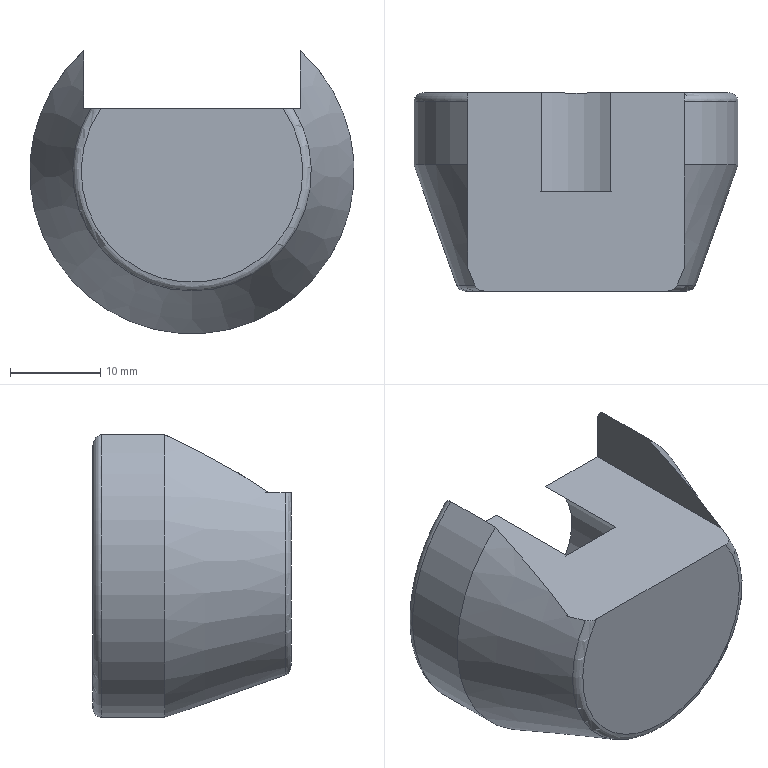Part | NX | features BREP 1 | 1 solid | 11 faces | box 36 x 22 x 31.416 mm | volume 12523 mm3 | plane 6 | torus 2 | cylinder 2 | cone 1 | commonest cylinder face diameters 16 x1 36 x1
STEP:
#1=CARTESIAN_POINT('',(-12.,-8.501,-23.));
#2=VERTEX_POINT('',#1);
#3=CARTESIAN_POINT('',(-11.235,-10.336,-23.));
#4=VERTEX_POINT('',#3);
#5=CARTESIAN_POINT('',(-12.,-8.501,-23.));
#6=CARTESIAN_POINT('',(-11.747,-9.114,-23.));
#7=CARTESIAN_POINT('',(-11.492,-9.726,-23.));
#8=CARTESIAN_POINT('',(-11.235,-10.336,-23.));
#9=B_SPLINE_CURVE_WITH_KNOTS('',3,(#5,#6,#7,#8),.UNSPECIFIED.,.F.,.F.,(4,4),(-0.01471,-0.01272),.UNSPECIFIED.);
#10=EDGE_CURVE('',#2,#4,#9,.T.);
#11=ORIENTED_EDGE('',*,*,#10,.T.);
#12=CARTESIAN_POINT('',(-10.108,-11.,-23.));
#13=VERTEX_POINT('',#12);
#14=CARTESIAN_POINT('',(-11.235,-10.336,-23.));
#15=CARTESIAN_POINT('',(-11.151,-10.535,-23.));
#16=CARTESIAN_POINT('',(-10.789,-10.903,-23.));
#17=CARTESIAN_POINT('',(-10.351,-11.,-23.));
#18=CARTESIAN_POINT('',(-10.108,-11.,-23.));
#19=B_SPLINE_CURVE_WITH_KNOTS('',3,(#14,#15,#16,#17,#18),.UNSPECIFIED.,.F.,.F.,(4,1,4),(0.,0.5,1.),.UNSPECIFIED.);
#20=EDGE_CURVE('',#13,#4,#19,.F.);
#21=ORIENTED_EDGE('',*,*,#20,.F.);
#22=CARTESIAN_POINT('',(10.108,-11.,-23.));
#23=VERTEX_POINT('',#22);
#24=CARTESIAN_POINT('',(0.,-11.,-23.));
#25=DIRECTION('',(1.,0.,0.));
#26=VECTOR('',#25,1000.);
#27=LINE('',#24,#26);
#28=EDGE_CURVE('',#13,#23,#27,.T.);
#29=ORIENTED_EDGE('',*,*,#28,.T.);
#30=CARTESIAN_POINT('',(11.235,-10.336,-23.));
#31=VERTEX_POINT('',#30);
#32=CARTESIAN_POINT('',(10.108,-11.,-23.));
#33=CARTESIAN_POINT('',(10.365,-11.,-23.));
#34=CARTESIAN_POINT('',(10.786,-10.9,-23.));
#35=CARTESIAN_POINT('',(11.151,-10.536,-23.));
#36=CARTESIAN_POINT('',(11.235,-10.336,-23.));
#37=B_SPLINE_CURVE_WITH_KNOTS('',3,(#32,#33,#34,#35,#36),.UNSPECIFIED.,.F.,.F.,(4,1,4),(0.,0.5,1.),.UNSPECIFIED.);
#38=EDGE_CURVE('',#31,#23,#37,.F.);
#39=ORIENTED_EDGE('',*,*,#38,.F.);
#40=CARTESIAN_POINT('',(12.,-8.501,-23.));
#41=VERTEX_POINT('',#40);
#42=CARTESIAN_POINT('',(11.235,-10.336,-23.));
#43=CARTESIAN_POINT('',(11.492,-9.726,-23.));
#44=CARTESIAN_POINT('',(11.747,-9.114,-23.));
#45=CARTESIAN_POINT('',(12.,-8.501,-23.));
#46=B_SPLINE_CURVE_WITH_KNOTS('',3,(#42,#43,#44,#45),.UNSPECIFIED.,.F.,.F.,(4,4),(0.01272,0.01471),.UNSPECIFIED.);
#47=EDGE_CURVE('',#31,#41,#46,.T.);
#48=ORIENTED_EDGE('',*,*,#47,.T.);
#49=CARTESIAN_POINT('',(12.,11.,-23.));
#50=VERTEX_POINT('',#49);
#51=CARTESIAN_POINT('',(12.,-60.,-23.));
#52=DIRECTION('',(0.,1.,0.));
#53=VECTOR('',#52,1000.);
#54=LINE('',#51,#53);
#55=EDGE_CURVE('',#41,#50,#54,.T.);
#56=ORIENTED_EDGE('',*,*,#55,.T.);
#57=CARTESIAN_POINT('',(3.873,11.,-23.));
#58=VERTEX_POINT('',#57);
#59=CARTESIAN_POINT('',(-12.,11.,-23.));
#60=DIRECTION('',(1.,0.,0.));
#61=VECTOR('',#60,1000.);
#62=LINE('',#59,#61);
#63=EDGE_CURVE('',#58,#50,#62,.T.);
#64=ORIENTED_EDGE('',*,*,#63,.F.);
#65=CARTESIAN_POINT('',(3.873,0.,-23.));
#66=VERTEX_POINT('',#65);
#67=CARTESIAN_POINT('',(3.873,71.,-23.));
#68=DIRECTION('',(0.,1.,0.));
#69=VECTOR('',#68,1000.);
#70=LINE('',#67,#69);
#71=EDGE_CURVE('',#66,#58,#70,.T.);
#72=ORIENTED_EDGE('',*,*,#71,.F.);
#73=CARTESIAN_POINT('',(-3.873,0.,-23.));
#74=VERTEX_POINT('',#73);
#75=CARTESIAN_POINT('',(0.,0.,-23.));
#76=DIRECTION('',(1.,0.,0.));
#77=VECTOR('',#76,1000.);
#78=LINE('',#75,#77);
#79=EDGE_CURVE('',#74,#66,#78,.T.);
#80=ORIENTED_EDGE('',*,*,#79,.F.);
#81=CARTESIAN_POINT('',(-3.873,11.,-23.));
#82=VERTEX_POINT('',#81);
#83=CARTESIAN_POINT('',(-3.873,71.,-23.));
#84=DIRECTION('',(0.,-1.,0.));
#85=VECTOR('',#84,1000.);
#86=LINE('',#83,#85);
#87=EDGE_CURVE('',#82,#74,#86,.T.);
#88=ORIENTED_EDGE('',*,*,#87,.F.);
#89=CARTESIAN_POINT('',(-12.,11.,-23.));
#90=VERTEX_POINT('',#89);
#91=CARTESIAN_POINT('',(-12.,11.,-23.));
#92=DIRECTION('',(1.,0.,0.));
#93=VECTOR('',#92,1000.);
#94=LINE('',#91,#93);
#95=EDGE_CURVE('',#90,#82,#94,.T.);
#96=ORIENTED_EDGE('',*,*,#95,.F.);
#97=CARTESIAN_POINT('',(-12.,-60.,-23.));
#98=DIRECTION('',(0.,1.,0.));
#99=VECTOR('',#98,1000.);
#100=LINE('',#97,#99);
#101=EDGE_CURVE('',#2,#90,#100,.T.);
#102=ORIENTED_EDGE('',*,*,#101,.F.);
#103=EDGE_LOOP('',(#11,#21,#29,#39,#48,#56,#64,#72,#80,#88,#96,#102));
#104=FACE_BOUND('',#103,.T.);
#105=CARTESIAN_POINT('',(-12.,-60.,-23.));
#106=DIRECTION('',(0.,0.,1.));
#107=DIRECTION('',(1.,0.,0.));
#108=AXIS2_PLACEMENT_3D('',#105,#106,#107);
#109=PLANE('',#108);
#110=ADVANCED_FACE('',(#104),#109,.T.);
#111=CARTESIAN_POINT('',(0.,-11.,-30.));
#112=DIRECTION('',(0.,1.,0.));
#113=DIRECTION('',(0.,0.,1.));
#114=AXIS2_PLACEMENT_3D('',#111,#112,#113);
#115=CIRCLE('',#114,12.295);
#116=EDGE_CURVE('',#23,#13,#115,.T.);
#117=ORIENTED_EDGE('',*,*,#116,.T.);
#118=ORIENTED_EDGE('',*,*,#20,.T.);
#119=CARTESIAN_POINT('',(0.,-10.336,-30.));
#120=DIRECTION('',(0.,1.,0.));
#121=DIRECTION('',(0.,0.,1.));
#122=AXIS2_PLACEMENT_3D('',#119,#120,#121);
#123=CIRCLE('',#122,13.237);
#124=EDGE_CURVE('',#31,#4,#123,.T.);
#125=ORIENTED_EDGE('',*,*,#124,.F.);
#126=ORIENTED_EDGE('',*,*,#38,.T.);
#127=EDGE_LOOP('',(#117,#118,#125,#126));
#128=FACE_BOUND('',#127,.T.);
#129=CARTESIAN_POINT('',(0.,-10.,-30.));
#130=DIRECTION('',(0.,1.,0.));
#131=DIRECTION('',(0.,0.,1.));
#132=AXIS2_PLACEMENT_3D('',#129,#130,#131);
#133=TOROIDAL_SURFACE('',#132,12.295,1.);
#134=ADVANCED_FACE('',(#128),#133,.T.);
#135=CARTESIAN_POINT('',(12.,3.,-16.584));
#136=VERTEX_POINT('',#135);
#137=CARTESIAN_POINT('',(12.,-8.501,-23.));
#138=CARTESIAN_POINT('',(12.,-7.748,-22.466));
#139=CARTESIAN_POINT('',(12.,-6.487,-21.64));
#140=CARTESIAN_POINT('',(12.,-4.749,-20.613));
#141=CARTESIAN_POINT('',(12.,-3.72,-20.03));
#142=CARTESIAN_POINT('',(12.,-2.821,-19.535));
#143=CARTESIAN_POINT('',(12.,-2.239,-19.222));
#144=CARTESIAN_POINT('',(12.,-1.313,-18.732));
#145=CARTESIAN_POINT('',(12.,0.3313,-17.884));
#146=CARTESIAN_POINT('',(12.,1.898,-17.112));
#147=CARTESIAN_POINT('',(12.,3.,-16.584));
#148=B_SPLINE_CURVE_WITH_KNOTS('',3,(#137,#138,#139,#140,#141,#142,#143,#144,#145,#146,#147),.UNSPECIFIED.,.F.,.F.,(4,1,1,1,1,1,1,1,4),(0.,0.25,0.375,0.4375,0.5,0.5625,0.625,0.75,1.),.UNSPECIFIED.);
#149=EDGE_CURVE('',#41,#136,#148,.T.);
#150=ORIENTED_EDGE('',*,*,#149,.F.);
#151=ORIENTED_EDGE('',*,*,#47,.F.);
#152=ORIENTED_EDGE('',*,*,#124,.T.);
#153=ORIENTED_EDGE('',*,*,#10,.F.);
#154=CARTESIAN_POINT('',(-12.,3.,-16.584));
#155=VERTEX_POINT('',#154);
#156=CARTESIAN_POINT('',(-12.,3.,-16.584));
#157=CARTESIAN_POINT('',(-12.,1.898,-17.112));
#158=CARTESIAN_POINT('',(-12.,0.3307,-17.884));
#159=CARTESIAN_POINT('',(-12.,-1.315,-18.733));
#160=CARTESIAN_POINT('',(-12.,-2.242,-19.224));
#161=CARTESIAN_POINT('',(-12.,-2.825,-19.537));
#162=CARTESIAN_POINT('',(-12.,-3.722,-20.031));
#163=CARTESIAN_POINT('',(-12.,-4.751,-20.614));
#164=CARTESIAN_POINT('',(-12.,-6.487,-21.641));
#165=CARTESIAN_POINT('',(-12.,-7.748,-22.466));
#166=CARTESIAN_POINT('',(-12.,-8.501,-23.));
#167=B_SPLINE_CURVE_WITH_KNOTS('',3,(#156,#157,#158,#159,#160,#161,#162,#163,#164,#165,#166),.UNSPECIFIED.,.F.,.F.,(4,1,1,1,1,1,1,1,4),(0.,0.25,0.375,0.4375,0.5,0.5625,0.625,0.75,1.),.UNSPECIFIED.);
#168=EDGE_CURVE('',#155,#2,#167,.T.);
#169=ORIENTED_EDGE('',*,*,#168,.F.);
#170=CARTESIAN_POINT('',(0.,3.,-30.));
#171=DIRECTION('',(0.,1.,0.));
#172=DIRECTION('',(0.,0.,1.));
#173=AXIS2_PLACEMENT_3D('',#170,#171,#172);
#174=CIRCLE('',#173,18.);
#175=EDGE_CURVE('',#136,#155,#174,.T.);
#176=ORIENTED_EDGE('',*,*,#175,.F.);
#177=EDGE_LOOP('',(#150,#151,#152,#153,#169,#176));
#178=FACE_BOUND('',#177,.T.);
#179=CARTESIAN_POINT('',(0.,-10.336,-30.));
#180=DIRECTION('',(0.,1.,0.));
#181=DIRECTION('',(0.,0.,1.));
#182=AXIS2_PLACEMENT_3D('',#179,#180,#181);
#183=CONICAL_SURFACE('',#182,13.237,0.343);
#184=ADVANCED_FACE('',(#178),#183,.T.);
#185=ORIENTED_EDGE('',*,*,#116,.F.);
#186=ORIENTED_EDGE('',*,*,#28,.F.);
#187=EDGE_LOOP('',(#185,#186));
#188=FACE_BOUND('',#187,.T.);
#189=CARTESIAN_POINT('',(0.,-11.,-30.));
#190=DIRECTION('',(0.,1.,0.));
#191=DIRECTION('',(1.,0.,0.));
#192=AXIS2_PLACEMENT_3D('',#189,#190,#191);
#193=PLANE('',#192);
#194=ADVANCED_FACE('',(#188),#193,.F.);
#195=CARTESIAN_POINT('',(12.,11.,-17.958));
#196=VERTEX_POINT('',#195);
#197=CARTESIAN_POINT('',(-12.,11.,-17.958));
#198=VERTEX_POINT('',#197);
#199=CARTESIAN_POINT('',(0.,11.,-30.));
#200=DIRECTION('',(0.,1.,0.));
#201=DIRECTION('',(0.,0.,1.));
#202=AXIS2_PLACEMENT_3D('',#199,#200,#201);
#203=CIRCLE('',#202,17.);
#204=EDGE_CURVE('',#196,#198,#203,.T.);
#205=ORIENTED_EDGE('',*,*,#204,.F.);
#206=CARTESIAN_POINT('',(12.,10.,-16.584));
#207=VERTEX_POINT('',#206);
#208=CARTESIAN_POINT('',(12.,10.,-16.584));
#209=CARTESIAN_POINT('',(12.,10.304,-16.584));
#210=CARTESIAN_POINT('',(12.,10.875,-17.015));
#211=CARTESIAN_POINT('',(12.,11.,-17.637));
#212=CARTESIAN_POINT('',(12.,11.,-17.958));
#213=B_SPLINE_CURVE_WITH_KNOTS('',3,(#208,#209,#210,#211,#212),.UNSPECIFIED.,.F.,.F.,(4,1,4),(0.,0.5,1.),.UNSPECIFIED.);
#214=EDGE_CURVE('',#196,#207,#213,.F.);
#215=ORIENTED_EDGE('',*,*,#214,.T.);
#216=CARTESIAN_POINT('',(-12.,10.,-16.584));
#217=VERTEX_POINT('',#216);
#218=CARTESIAN_POINT('',(0.,10.,-30.));
#219=DIRECTION('',(0.,1.,0.));
#220=DIRECTION('',(0.,0.,1.));
#221=AXIS2_PLACEMENT_3D('',#218,#219,#220);
#222=CIRCLE('',#221,18.);
#223=EDGE_CURVE('',#207,#217,#222,.T.);
#224=ORIENTED_EDGE('',*,*,#223,.T.);
#225=CARTESIAN_POINT('',(-12.,11.,-17.958));
#226=CARTESIAN_POINT('',(-12.,11.,-17.638));
#227=CARTESIAN_POINT('',(-12.,10.875,-17.017));
#228=CARTESIAN_POINT('',(-12.,10.307,-16.584));
#229=CARTESIAN_POINT('',(-12.,10.,-16.584));
#230=B_SPLINE_CURVE_WITH_KNOTS('',3,(#225,#226,#227,#228,#229),.UNSPECIFIED.,.F.,.F.,(4,1,4),(0.,0.5,1.),.UNSPECIFIED.);
#231=EDGE_CURVE('',#217,#198,#230,.F.);
#232=ORIENTED_EDGE('',*,*,#231,.T.);
#233=EDGE_LOOP('',(#205,#215,#224,#232));
#234=FACE_BOUND('',#233,.T.);
#235=CARTESIAN_POINT('',(0.,10.,-30.));
#236=DIRECTION('',(0.,1.,0.));
#237=DIRECTION('',(0.,0.,1.));
#238=AXIS2_PLACEMENT_3D('',#235,#236,#237);
#239=TOROIDAL_SURFACE('',#238,17.,1.);
#240=ADVANCED_FACE('',(#234),#239,.T.);
#241=ORIENTED_EDGE('',*,*,#79,.T.);
#242=CARTESIAN_POINT('',(0.,0.,-30.));
#243=DIRECTION('',(0.,1.,0.));
#244=DIRECTION('',(0.,0.,1.));
#245=AXIS2_PLACEMENT_3D('',#242,#243,#244);
#246=CIRCLE('',#245,8.);
#247=EDGE_CURVE('',#66,#74,#246,.T.);
#248=ORIENTED_EDGE('',*,*,#247,.T.);
#249=EDGE_LOOP('',(#241,#248));
#250=FACE_BOUND('',#249,.T.);
#251=CARTESIAN_POINT('',(0.,0.,-30.));
#252=DIRECTION('',(0.,1.,0.));
#253=DIRECTION('',(1.,0.,0.));
#254=AXIS2_PLACEMENT_3D('',#251,#252,#253);
#255=PLANE('',#254);
#256=ADVANCED_FACE('',(#250),#255,.T.);
#257=ORIENTED_EDGE('',*,*,#247,.F.);
#258=ORIENTED_EDGE('',*,*,#71,.T.);
#259=CARTESIAN_POINT('',(0.,11.,-30.));
#260=DIRECTION('',(0.,1.,0.));
#261=DIRECTION('',(0.,0.,1.));
#262=AXIS2_PLACEMENT_3D('',#259,#260,#261);
#263=CIRCLE('',#262,8.);
#264=EDGE_CURVE('',#58,#82,#263,.T.);
#265=ORIENTED_EDGE('',*,*,#264,.T.);
#266=ORIENTED_EDGE('',*,*,#87,.T.);
#267=EDGE_LOOP('',(#257,#258,#265,#266));
#268=FACE_BOUND('',#267,.T.);
#269=CARTESIAN_POINT('',(0.,71.,-30.));
#270=DIRECTION('',(0.,-1.,0.));
#271=DIRECTION('',(0.,0.,1.));
#272=AXIS2_PLACEMENT_3D('',#269,#270,#271);
#273=CYLINDRICAL_SURFACE('',#272,8.);
#274=ADVANCED_FACE('',(#268),#273,.F.);
#275=CARTESIAN_POINT('',(12.,11.,-23.));
#276=DIRECTION('',(0.,0.,1.));
#277=VECTOR('',#276,1000.);
#278=LINE('',#275,#277);
#279=EDGE_CURVE('',#50,#196,#278,.T.);
#280=ORIENTED_EDGE('',*,*,#279,.T.);
#281=ORIENTED_EDGE('',*,*,#204,.T.);
#282=CARTESIAN_POINT('',(-12.,11.,-14.));
#283=DIRECTION('',(0.,0.,-1.));
#284=VECTOR('',#283,1000.);
#285=LINE('',#282,#284);
#286=EDGE_CURVE('',#198,#90,#285,.T.);
#287=ORIENTED_EDGE('',*,*,#286,.T.);
#288=ORIENTED_EDGE('',*,*,#95,.T.);
#289=ORIENTED_EDGE('',*,*,#264,.F.);
#290=ORIENTED_EDGE('',*,*,#63,.T.);
#291=EDGE_LOOP('',(#280,#281,#287,#288,#289,#290));
#292=FACE_BOUND('',#291,.T.);
#293=CARTESIAN_POINT('',(0.,11.,-13.));
#294=DIRECTION('',(0.,-1.,0.));
#295=DIRECTION('',(0.,0.,-1.));
#296=AXIS2_PLACEMENT_3D('',#293,#294,#295);
#297=PLANE('',#296);
#298=ADVANCED_FACE('',(#292),#297,.F.);
#299=CARTESIAN_POINT('',(12.,71.,-16.584));
#300=DIRECTION('',(0.,1.,0.));
#301=VECTOR('',#300,1000.);
#302=LINE('',#299,#301);
#303=EDGE_CURVE('',#136,#207,#302,.T.);
#304=ORIENTED_EDGE('',*,*,#303,.F.);
#305=ORIENTED_EDGE('',*,*,#175,.T.);
#306=CARTESIAN_POINT('',(-12.,71.,-16.584));
#307=DIRECTION('',(0.,-1.,0.));
#308=VECTOR('',#307,1000.);
#309=LINE('',#306,#308);
#310=EDGE_CURVE('',#217,#155,#309,.T.);
#311=ORIENTED_EDGE('',*,*,#310,.F.);
#312=ORIENTED_EDGE('',*,*,#223,.F.);
#313=EDGE_LOOP('',(#304,#305,#311,#312));
#314=FACE_BOUND('',#313,.T.);
#315=CARTESIAN_POINT('',(0.,71.,-30.));
#316=DIRECTION('',(0.,-1.,0.));
#317=DIRECTION('',(0.,0.,1.));
#318=AXIS2_PLACEMENT_3D('',#315,#316,#317);
#319=CYLINDRICAL_SURFACE('',#318,18.);
#320=ADVANCED_FACE('',(#314),#319,.T.);
#321=ORIENTED_EDGE('',*,*,#149,.T.);
#322=ORIENTED_EDGE('',*,*,#303,.T.);
#323=ORIENTED_EDGE('',*,*,#214,.F.);
#324=ORIENTED_EDGE('',*,*,#279,.F.);
#325=ORIENTED_EDGE('',*,*,#55,.F.);
#326=EDGE_LOOP('',(#321,#322,#323,#324,#325));
#327=FACE_BOUND('',#326,.T.);
#328=CARTESIAN_POINT('',(12.,-60.,-23.));
#329=DIRECTION('',(-1.,0.,0.));
#330=DIRECTION('',(0.,0.,1.));
#331=AXIS2_PLACEMENT_3D('',#328,#329,#330);
#332=PLANE('',#331);
#333=ADVANCED_FACE('',(#327),#332,.T.);
#334=ORIENTED_EDGE('',*,*,#168,.T.);
#335=ORIENTED_EDGE('',*,*,#101,.T.);
#336=ORIENTED_EDGE('',*,*,#286,.F.);
#337=ORIENTED_EDGE('',*,*,#231,.F.);
#338=ORIENTED_EDGE('',*,*,#310,.T.);
#339=EDGE_LOOP('',(#334,#335,#336,#337,#338));
#340=FACE_BOUND('',#339,.T.);
#341=CARTESIAN_POINT('',(-12.,-60.,-14.));
#342=DIRECTION('',(1.,0.,0.));
#343=DIRECTION('',(0.,1.,0.));
#344=AXIS2_PLACEMENT_3D('',#341,#342,#343);
#345=PLANE('',#344);
#346=ADVANCED_FACE('',(#340),#345,.T.);
#347=CLOSED_SHELL('',(#110,#134,#184,#194,#240,#256,#274,#298,#320,#333,#346));
#348=MANIFOLD_SOLID_BREP('',#347);
#349=(LENGTH_UNIT()NAMED_UNIT(*)SI_UNIT(.MILLI.,.METRE.));
#350=UNCERTAINTY_MEASURE_WITH_UNIT(LENGTH_MEASURE(0.0508),#349,'','');
#351=(NAMED_UNIT(*)PLANE_ANGLE_UNIT()SI_UNIT($,.RADIAN.));
#352=(NAMED_UNIT(*)SI_UNIT($,.STERADIAN.)SOLID_ANGLE_UNIT());
#353=(GEOMETRIC_REPRESENTATION_CONTEXT(3)GLOBAL_UNCERTAINTY_ASSIGNED_CONTEXT((#350))GLOBAL_UNIT_ASSIGNED_CONTEXT((#349,#351,#352))REPRESENTATION_CONTEXT('',''));
#354=ADVANCED_BREP_SHAPE_REPRESENTATION('',(#348),#353);